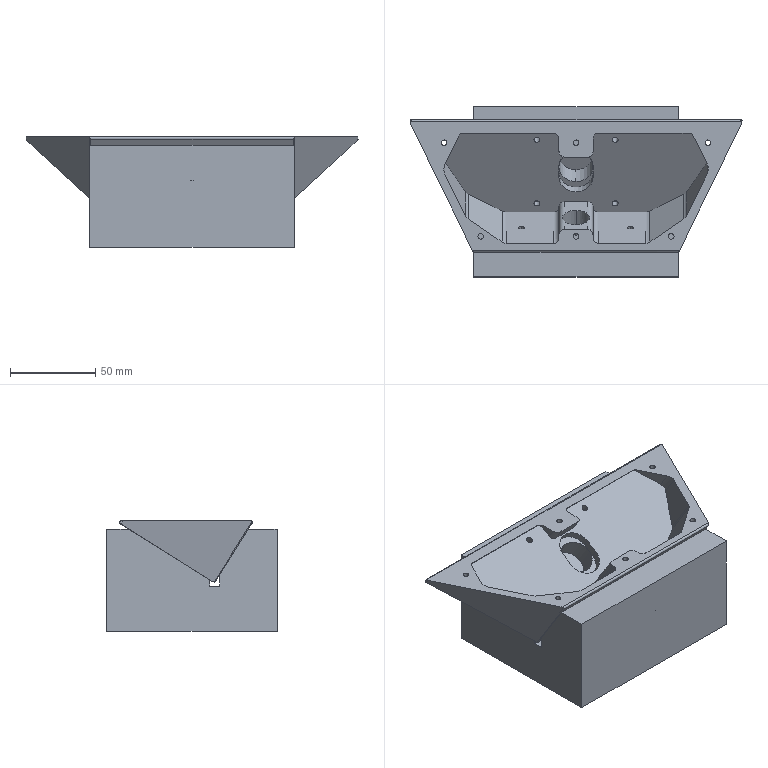NC program | Mastercam | posted with a generic post | part box 195.124 x 100 x 65 mm
Lines 1 to 1369 of 1918, first 1278 of 1369 lines:
%
O0000()
(MATERIAL - ALUMINUM MM - 2024)
( T1 | 16 RC | H1 | D1 | WEAR COMP | TOOL DIA. - 16. | XY STOCK TO LEAVE - -3. | Z STOCK TO LEAVE - .1 )
( T2 | 16 FI | H2 | D2 | WEAR COMP | TOOL DIA. - 16. | XY STOCK TO LEAVE - -3. | Z STOCK TO LEAVE - 0. )
( T3 | 6 SPD | H3 )
( T4 | 3.3 DR | H4 )
( T5 | 3.2 DR | H5 )
( T6 | 2.5 FEM | H6 | D6 | WEAR COMP | TOOL DIA. - 2.5 | XY STOCK TO LEAVE - -.015 | Z STOCK TO LEAVE - 0. )
( T7 | 3.15 THML | H7 | D7 | WEAR COMP | TOOL DIA. - 3.15 )
( T11 | 3.5 DR | H11 )
N100 G21
N110 G0 G17 G40 G49 G80 G90
N120 T1 M6
N130 G0 G90 G54 X-86.736 Y-13.812 A0. S2300 M3
N140 G43 H1 Z50.
N150 Z36.439
N160 G1 Z.1 F2000.
N170 G41 D1 X-75.958 Y-8.535 F3000.
N180 G3 X-75.509 Y-7.816 I-.352 J.719
N190 G1 X-75.53 Y-7.636
N200 X-75.591 Y-7.464
N210 X-81.561 Y4.728
N220 X-82.05 Y5.913
N230 X-82.43 Y7.304
N240 X-82.637 Y8.729
N250 X-82.672 Y10.164
N260 X-82.534 Y11.588
N270 X-82.229 Y12.977
N280 X-81.788 Y14.23
N290 X-81.522 Y14.815
N300 X-73.284 Y31.64
N310 X-72.634 Y32.725
N320 X-71.667 Y33.84
N330 X-70.515 Y34.764
N340 X-69.209 Y35.459
N350 X-67.795 Y35.893
N360 X-66.565 Y36.019
N370 X-12.744 Y36.02
N380 X-11.467 Y35.889
N390 X-10.017 Y35.434
N400 X-8.708 Y34.72
N410 X-7.575 Y33.794
N420 X-6.639 Y32.702
N430 X-5.911 Y31.486
N440 X-5.393 Y30.185
N450 X-5.086 Y28.835
N460 X-5. Y27.667
N470 Y21.868
N480 X5.
N490 Y27.683
N500 X5.102 Y28.951
N510 X5.452 Y30.375
N520 X6.028 Y31.717
N530 X6.817 Y32.942
N540 X7.807 Y34.013
N550 X8.974 Y34.891
N560 X10.285 Y35.541
N570 X11.67 Y35.923
N580 X12.783 Y36.02
N590 X66.704
N600 X67.965 Y35.892
N610 X69.4 Y35.448
N620 X70.699 Y34.749
N630 X71.827 Y33.841
N640 X72.762 Y32.769
N650 X73.401 Y31.728
N660 X81.643 Y14.901
N670 X82.132 Y13.716
N680 X82.512 Y12.324
N690 X82.719 Y10.899
N700 X82.753 Y9.464
N710 X82.616 Y8.04
N720 X82.31 Y6.651
N730 X81.87 Y5.399
N740 X81.603 Y4.813
N750 X69.621 Y-19.658
N760 X68.987 Y-20.768
N770 X68.12 Y-21.904
N780 X67.136 Y-22.885
N790 X66.307 Y-23.523
N800 X46.099 Y-37.28
N810 X45.017 Y-37.907
N820 X43.691 Y-38.431
N830 X42.312 Y-38.746
N840 X41.122 Y-38.835
N850 X12.744
N860 X11.467 Y-38.703
N870 X10.017 Y-38.248
N880 X8.708 Y-37.535
N890 X7.575 Y-36.609
N900 X6.639 Y-35.517
N910 X5.911 Y-34.301
N920 X5.393 Y-33.
N930 X5.086 Y-31.65
N940 X5.007 Y-30.58
N950 X-5.007
N960 X-5.102 Y-31.766
N970 X-5.452 Y-33.189
N980 X-6.028 Y-34.531
N990 X-6.817 Y-35.756
N1000 X-7.807 Y-36.827
N1010 X-8.974 Y-37.706
N1020 X-10.285 Y-38.355
N1030 X-11.67 Y-38.738
N1040 X-12.783 Y-38.835
N1050 X-41.13
N1060 X-42.359 Y-38.739
N1070 X-43.741 Y-38.415
N1080 X-45.049 Y-37.891
N1090 X-46.104 Y-37.278
N1100 X-66.333 Y-23.505
N1110 X-67.302 Y-22.739
N1120 X-68.278 Y-21.718
N1130 X-69.095 Y-20.598
N1140 X-69.633 Y-19.636
N1150 X-75.812 Y-7.016
N1160 G3 X-76.53 Y-6.568 I-.718 J-.351
N1170 X-76.882 Y-6.649 I0. J-.799
N1180 G1 G40 X-87.659 Y-11.926
N1190 G0 Z50.
N1200 X-63.18 Y.421
N1210 Z36.439
N1220 G1 Z.1 F2000.
N1230 G41 D1 X-73.958 Y-4.856 F3000.
N1240 G3 X-74.406 Y-5.574 I.352 J-.718
N1250 X-74.325 Y-5.926 I.8 J0.
N1260 G1 X-59.636 Y-35.926
N1270 X59.636
N1280 X94.816 Y35.926
N1290 X-94.816
N1300 X-74.105 Y-6.375
N1310 G3 X-73.386 Y-6.824 I.719 J.352
N1320 X-73.034 Y-6.742 I0. J.801
N1330 G1 G40 X-62.257 Y-1.465
N1340 G0 Z50.
N1350 M5
N1360 G91 G28 Z0.
N1370 A0.
N1380 M01
N1390 T2 M6
N1400 G0 G90 G17 G54 X-86.736 Y-13.812 A0. S4000 M3
N1410 G43 H2 Z50.
N1420 Z36.439
N1430 G1 Z0. F2000.
N1440 G41 D2 X-75.958 Y-8.535 F800.
N1450 G3 X-75.509 Y-7.816 I-.352 J.719
N1460 G1 X-75.53 Y-7.636
N1470 X-75.591 Y-7.464
N1480 X-81.561 Y4.728
N1490 X-82.05 Y5.913
N1500 X-82.43 Y7.304
N1510 X-82.637 Y8.729
N1520 X-82.672 Y10.164
N1530 X-82.534 Y11.588
N1540 X-82.229 Y12.977
N1550 X-81.788 Y14.23
N1560 X-81.522 Y14.815
N1570 X-73.284 Y31.64
N1580 X-72.634 Y32.725
N1590 X-71.667 Y33.84
N1600 X-70.515 Y34.764
N1610 X-69.209 Y35.459
N1620 X-67.795 Y35.893
N1630 X-66.565 Y36.019
N1640 X-12.744 Y36.02
N1650 X-11.467 Y35.889
N1660 X-10.017 Y35.434
N1670 X-8.708 Y34.72
N1680 X-7.575 Y33.794
N1690 X-6.639 Y32.702
N1700 X-5.911 Y31.486
N1710 X-5.393 Y30.185
N1720 X-5.086 Y28.835
N1730 X-5. Y27.667
N1740 Y21.868
N1750 X5.
N1760 Y27.683
N1770 X5.102 Y28.951
N1780 X5.452 Y30.375
N1790 X6.028 Y31.717
N1800 X6.817 Y32.942
N1810 X7.807 Y34.013
N1820 X8.974 Y34.891
N1830 X10.285 Y35.541
N1840 X11.67 Y35.923
N1850 X12.783 Y36.02
N1860 X66.704
N1870 X67.965 Y35.892
N1880 X69.4 Y35.448
N1890 X70.699 Y34.749
N1900 X71.827 Y33.841
N1910 X72.762 Y32.769
N1920 X73.401 Y31.728
N1930 X81.643 Y14.901
N1940 X82.132 Y13.716
N1950 X82.512 Y12.324
N1960 X82.719 Y10.899
N1970 X82.753 Y9.464
N1980 X82.616 Y8.04
N1990 X82.31 Y6.651
N2000 X81.87 Y5.399
N2010 X81.603 Y4.813
N2020 X69.621 Y-19.658
N2030 X68.987 Y-20.768
N2040 X68.12 Y-21.904
N2050 X67.136 Y-22.885
N2060 X66.307 Y-23.523
N2070 X46.099 Y-37.28
N2080 X45.017 Y-37.907
N2090 X43.691 Y-38.431
N2100 X42.312 Y-38.746
N2110 X41.122 Y-38.835
N2120 X12.744
N2130 X11.467 Y-38.703
N2140 X10.017 Y-38.248
N2150 X8.708 Y-37.535
N2160 X7.575 Y-36.609
N2170 X6.639 Y-35.517
N2180 X5.911 Y-34.301
N2190 X5.393 Y-33.
N2200 X5.086 Y-31.65
N2210 X5.007 Y-30.58
N2220 X-5.007
N2230 X-5.102 Y-31.766
N2240 X-5.452 Y-33.189
N2250 X-6.028 Y-34.531
N2260 X-6.817 Y-35.756
N2270 X-7.807 Y-36.827
N2280 X-8.974 Y-37.706
N2290 X-10.285 Y-38.355
N2300 X-11.67 Y-38.738
N2310 X-12.783 Y-38.835
N2320 X-41.13
N2330 X-42.359 Y-38.739
N2340 X-43.741 Y-38.415
N2350 X-45.049 Y-37.891
N2360 X-46.104 Y-37.278
N2370 X-66.333 Y-23.505
N2380 X-67.302 Y-22.739
N2390 X-68.278 Y-21.718
N2400 X-69.095 Y-20.598
N2410 X-69.633 Y-19.636
N2420 X-75.812 Y-7.016
N2430 G3 X-76.53 Y-6.568 I-.718 J-.351
N2440 X-76.882 Y-6.649 I0. J-.799
N2450 G1 G40 X-87.659 Y-11.926
N2460 G0 Z50.
N2470 X-63.18 Y.421
N2480 Z36.439
N2490 G1 Z0. F2000.
N2500 G41 D2 X-73.958 Y-4.856 F800.
N2510 G3 X-74.406 Y-5.574 I.352 J-.718
N2520 X-74.325 Y-5.926 I.8 J0.
N2530 G1 X-59.636 Y-35.926
N2540 X59.636
N2550 X94.816 Y35.926
N2560 X-94.816
N2570 X-74.105 Y-6.375
N2580 G3 X-73.386 Y-6.824 I.719 J.352
N2590 X-73.034 Y-6.742 I0. J.801
N2600 G1 G40 X-62.257 Y-1.465
N2610 G0 Z50.
N2620 M5
N2630 G91 G28 Z0.
N2640 A0.
N2650 M01
N2660 T3 M6
N2670 G0 G90 G17 G54 X77.5 Y25.269 A0. S2000 M3
N2680 G43 H3 Z50.
N2690 G98 G81 Z-2. R1. F100.
N2700 X0.
N2710 X-77.5
N2720 X-56. Y-29.731
N2730 X0.
N2740 X56.
N2750 G80
N2760 M5
N2770 G91 G0 G28 Z0.
N2780 A0.
N2790 M01
N2800 T4 M6
N2810 G0 G90 G17 G54 X56. Y-29.731 A0. S1200 M3
N2820 G43 H4 Z50.
N2830 G98 G83 Z-8. R1. Q3. F100.
N2840 X-56.
N2850 G80
N2860 G0 X77.5 Y25.269
N2870 G98 G83 Z-7.5 R1. Q3. F100.
N2880 X-77.5
N2890 G80
N2900 M5
N2910 G91 G0 G28 Z0.
N2920 A0.
N2930 M01
N2940 T5 M6
N2950 G0 G90 G17 G54 X0. Y-29.731 A0. S1200 M3
N2960 G43 H5 Z50.
N2970 G98 G81 Z-8. R1. F100.
N2980 Y25.269
N2990 G80
N3000 G0 Y-29.731
N3010 G98 G81 Z-8. R1. F100.
N3020 Y25.269
N3030 G80
N3040 M5
N3050 G91 G0 G28 Z0.
N3060 A0.
N3070 M01
N3080 T6 M6
N3090 G0 G90 G17 G54 X0. Y-29.731 A0. S3500 M3
N3100 G43 H6 Z50.
N3110 Z2.
N3120 G1 Z-6. F600.
N3130 G41 D6 X.39 F100.
N3140 G3 X.403 Y-29.66 I-.195 J.071
N3150 X.39 Y-29.589 I-.208 J0.
N3160 X0. Y-29.316 I-.39 J-.142
N3170 X-.415 Y-29.731 I0. J-.415
N3180 X0. Y-30.146 I.415 J0.
N3190 X.415 Y-29.731 I0. J.415
N3200 X.39 Y-29.589 I-.415 J0.
N3210 X.331 Y-29.48 I-.39 J-.142
N3220 X.211 Y-29.403 I-.166 J-.125
N3230 G1 G40 X0. Y-29.731
N3240 G41 D6 X.39
N3250 G3 X.403 Y-29.66 I-.195 J.071
N3260 X.39 Y-29.589 I-.208 J0.
N3270 X0. Y-29.316 I-.39 J-.142
N3280 X-.415 Y-29.731 I0. J-.415
N3290 X0. Y-30.146 I.415 J0.
N3300 X.415 Y-29.731 I0. J.415
N3310 X.39 Y-29.589 I-.415 J0.
N3320 X.331 Y-29.48 I-.39 J-.142
N3330 X.211 Y-29.403 I-.166 J-.125
N3340 G1 G40 X0. Y-29.731
N3350 G0 Z50.
N3360 Y25.269
N3370 Z2.
N3380 G1 Z-6. F600.
N3390 G41 D6 X.39 F100.
N3400 G3 X.403 Y25.34 I-.195 J.071
N3410 X.39 Y25.411 I-.208 J0.
N3420 X0. Y25.684 I-.39 J-.142
N3430 X-.415 Y25.269 I0. J-.415
N3440 X0. Y24.854 I.415 J0.
N3450 X.415 Y25.269 I0. J.415
N3460 X.39 Y25.411 I-.415 J0.
N3470 X.331 Y25.52 I-.39 J-.142
N3480 X.211 Y25.597 I-.166 J-.125
N3490 G1 G40 X0. Y25.269
N3500 G41 D6 X.39
N3510 G3 X.403 Y25.34 I-.195 J.071
N3520 X.39 Y25.411 I-.208 J0.
N3530 X0. Y25.684 I-.39 J-.142
N3540 X-.415 Y25.269 I0. J-.415
N3550 X0. Y24.854 I.415 J0.
N3560 X.415 Y25.269 I0. J.415
N3570 X.39 Y25.411 I-.415 J0.
N3580 X.331 Y25.52 I-.39 J-.142
N3590 X.211 Y25.597 I-.166 J-.125
N3600 G1 G40 X0. Y25.269
N3610 G0 Z50.
N3620 M5
N3630 G91 G28 Z0.
N3640 A0.
N3650 M01
N3660 T7 M6
N3670 G0 G90 G17 G54 X56. Y-29.731 A0. S3000 M3
N3680 G43 H7 Z50.
N3690 Z2.
N3700 G1 Z-5.5 F600.
N3710 G41 D7 Y-29.891 F200.
N3720 G3 X56.16 Y-29.731 Z-5.325 I0. J.16
N3730 X56. Y-29.571 Z-5.15 I-.16 J0.
N3740 X55.84 Y-29.731 Z-4.975 I0. J-.16
N3750 X56. Y-29.891 Z-4.8 I.16 J0.
N3760 X56.16 Y-29.731 Z-4.625 I0. J.16
N3770 X56. Y-29.571 Z-4.45 I-.16 J0.
N3780 G1 G40 Y-29.731
N3790 Z-3.4 F600.
N3800 G41 D7 Y-29.891 F200.
N3810 G3 X56.16 Y-29.731 Z-3.225 I0. J.16
N3820 X56. Y-29.571 Z-3.05 I-.16 J0.
N3830 X55.84 Y-29.731 Z-2.875 I0. J-.16
N3840 X56. Y-29.891 Z-2.7 I.16 J0.
N3850 X56.16 Y-29.731 Z-2.525 I0. J.16
N3860 X56. Y-29.571 Z-2.35 I-.16 J0.
N3870 G1 G40 Y-29.731
N3880 Z-1.3 F600.
N3890 G41 D7 Y-29.891 F200.
N3900 G3 X56.16 Y-29.731 Z-1.125 I0. J.16
N3910 X56. Y-29.571 Z-.95 I-.16 J0.
N3920 X55.84 Y-29.731 Z-.775 I0. J-.16
N3930 X56. Y-29.891 Z-.6 I.16 J0.
N3940 X56.16 Y-29.731 Z-.425 I0. J.16
N3950 X56. Y-29.571 Z-.25 I-.16 J0.
N3960 G1 G40 Y-29.731
N3970 Z-5.5 F600.
N3980 G41 D7 Y-29.956 F200.
N3990 G3 X56.225 Y-29.731 Z-5.325 I0. J.225
N4000 X56. Y-29.506 Z-5.15 I-.225 J0.
N4010 X55.775 Y-29.731 Z-4.975 I0. J-.225
N4020 X56. Y-29.956 Z-4.8 I.225 J0.
N4030 X56.225 Y-29.731 Z-4.625 I0. J.225
N4040 X56. Y-29.506 Z-4.45 I-.225 J0.
N4050 G1 G40 Y-29.731
N4060 Z-3.4 F600.
N4070 G41 D7 Y-29.956 F200.
N4080 G3 X56.225 Y-29.731 Z-3.225 I0. J.225
N4090 X56. Y-29.506 Z-3.05 I-.225 J0.
N4100 X55.775 Y-29.731 Z-2.875 I0. J-.225
N4110 X56. Y-29.956 Z-2.7 I.225 J0.
N4120 X56.225 Y-29.731 Z-2.525 I0. J.225
N4130 X56. Y-29.506 Z-2.35 I-.225 J0.
N4140 G1 G40 Y-29.731
N4150 Z-1.3 F600.
N4160 G41 D7 Y-29.956 F200.
N4170 G3 X56.225 Y-29.731 Z-1.125 I0. J.225
N4180 X56. Y-29.506 Z-.95 I-.225 J0.
N4190 X55.775 Y-29.731 Z-.775 I0. J-.225
N4200 X56. Y-29.956 Z-.6 I.225 J0.
N4210 X56.225 Y-29.731 Z-.425 I0. J.225
N4220 X56. Y-29.506 Z-.25 I-.225 J0.
N4230 G1 G40 Y-29.731
N4240 Z-5.5 F600.
N4250 G41 D7 Y-30.021 F200.
N4260 G3 X56.29 Y-29.731 Z-5.325 I0. J.29
N4270 X56. Y-29.441 Z-5.15 I-.29 J0.
N4280 X55.71 Y-29.731 Z-4.975 I0. J-.29
N4290 X56. Y-30.021 Z-4.8 I.29 J0.
N4300 X56.29 Y-29.731 Z-4.625 I0. J.29
N4310 X56. Y-29.441 Z-4.45 I-.29 J0.
N4320 G1 G40 Y-29.731
N4330 Z-3.4 F600.
N4340 G41 D7 Y-30.021 F200.
N4350 G3 X56.29 Y-29.731 Z-3.225 I0. J.29
N4360 X56. Y-29.441 Z-3.05 I-.29 J0.
N4370 X55.71 Y-29.731 Z-2.875 I0. J-.29
N4380 X56. Y-30.021 Z-2.7 I.29 J0.
N4390 X56.29 Y-29.731 Z-2.525 I0. J.29
N4400 X56. Y-29.441 Z-2.35 I-.29 J0.
N4410 G1 G40 Y-29.731
N4420 Z-1.3 F600.
N4430 G41 D7 Y-30.021 F200.
N4440 G3 X56.29 Y-29.731 Z-1.125 I0. J.29
N4450 X56. Y-29.441 Z-.95 I-.29 J0.
N4460 X55.71 Y-29.731 Z-.775 I0. J-.29
N4470 X56. Y-30.021 Z-.6 I.29 J0.
N4480 X56.29 Y-29.731 Z-.425 I0. J.29
N4490 X56. Y-29.441 Z-.25 I-.29 J0.
N4500 G1 G40 Y-29.731
N4510 Z-5.5 F600.
N4520 G41 D7 Y-30.086 F200.
N4530 G3 X56.355 Y-29.731 Z-5.325 I0. J.355
N4540 X56. Y-29.376 Z-5.15 I-.355 J0.
N4550 X55.645 Y-29.731 Z-4.975 I0. J-.355
N4560 X56. Y-30.086 Z-4.8 I.355 J0.
N4570 X56.355 Y-29.731 Z-4.625 I0. J.355
N4580 X56. Y-29.376 Z-4.45 I-.355 J0.
N4590 G1 G40 Y-29.731
N4600 Z-3.4 F600.
N4610 G41 D7 Y-30.086 F200.
N4620 G3 X56.355 Y-29.731 Z-3.225 I0. J.355
N4630 X56. Y-29.376 Z-3.05 I-.355 J0.
N4640 X55.645 Y-29.731 Z-2.875 I0. J-.355
N4650 X56. Y-30.086 Z-2.7 I.355 J0.
N4660 X56.355 Y-29.731 Z-2.525 I0. J.355
N4670 X56. Y-29.376 Z-2.35 I-.355 J0.
N4680 G1 G40 Y-29.731
N4690 Z-1.3 F600.
N4700 G41 D7 Y-30.086 F200.
N4710 G3 X56.355 Y-29.731 Z-1.125 I0. J.355
N4720 X56. Y-29.376 Z-.95 I-.355 J0.
N4730 X55.645 Y-29.731 Z-.775 I0. J-.355
N4740 X56. Y-30.086 Z-.6 I.355 J0.
N4750 X56.355 Y-29.731 Z-.425 I0. J.355
N4760 X56. Y-29.376 Z-.25 I-.355 J0.
N4770 G1 G40 Y-29.731
N4780 Z-5.5 F600.
N4790 G41 D7 Y-30.151 F200.
N4800 G3 X56.42 Y-29.731 Z-5.325 I0. J.42
N4810 X56. Y-29.311 Z-5.15 I-.42 J0.
N4820 X55.58 Y-29.731 Z-4.975 I0. J-.42
N4830 X56. Y-30.151 Z-4.8 I.42 J0.
N4840 X56.42 Y-29.731 Z-4.625 I0. J.42
N4850 X56. Y-29.311 Z-4.45 I-.42 J0.
N4860 G1 G40 Y-29.731
N4870 Z-3.4 F600.
N4880 G41 D7 Y-30.151 F200.
N4890 G3 X56.42 Y-29.731 Z-3.225 I0. J.42
N4900 X56. Y-29.311 Z-3.05 I-.42 J0.
N4910 X55.58 Y-29.731 Z-2.875 I0. J-.42
N4920 X56. Y-30.151 Z-2.7 I.42 J0.
N4930 X56.42 Y-29.731 Z-2.525 I0. J.42
N4940 X56. Y-29.311 Z-2.35 I-.42 J0.
N4950 G1 G40 Y-29.731
N4960 Z-1.3 F600.
N4970 G41 D7 Y-30.151 F200.
N4980 G3 X56.42 Y-29.731 Z-1.125 I0. J.42
N4990 X56. Y-29.311 Z-.95 I-.42 J0.
N5000 X55.58 Y-29.731 Z-.775 I0. J-.42
N5010 X56. Y-30.151 Z-.6 I.42 J0.
N5020 X56.42 Y-29.731 Z-.425 I0. J.42
N5030 X56. Y-29.311 Z-.25 I-.42 J0.
N5040 G1 G40 Y-29.731
N5050 Z-5.5 F600.
N5060 G41 D7 Y-30.156 F200.
N5070 G3 X56.425 Y-29.731 Z-5.325 I0. J.425
N5080 X56. Y-29.306 Z-5.15 I-.425 J0.
N5090 X55.575 Y-29.731 Z-4.975 I0. J-.425
N5100 X56. Y-30.156 Z-4.8 I.425 J0.
N5110 X56.425 Y-29.731 Z-4.625 I0. J.425
N5120 X56. Y-29.306 Z-4.45 I-.425 J0.
N5130 G1 G40 Y-29.731
N5140 Z-3.4 F600.
N5150 G41 D7 Y-30.156 F200.
N5160 G3 X56.425 Y-29.731 Z-3.225 I0. J.425
N5170 X56. Y-29.306 Z-3.05 I-.425 J0.
N5180 X55.575 Y-29.731 Z-2.875 I0. J-.425
N5190 X56. Y-30.156 Z-2.7 I.425 J0.
N5200 X56.425 Y-29.731 Z-2.525 I0. J.425
N5210 X56. Y-29.306 Z-2.35 I-.425 J0.
N5220 G1 G40 Y-29.731
N5230 Z-1.3 F600.
N5240 G41 D7 Y-30.156 F200.
N5250 G3 X56.425 Y-29.731 Z-1.125 I0. J.425
N5260 X56. Y-29.306 Z-.95 I-.425 J0.
N5270 X55.575 Y-29.731 Z-.775 I0. J-.425
N5280 X56. Y-30.156 Z-.6 I.425 J0.
N5290 X56.425 Y-29.731 Z-.425 I0. J.425
N5300 X56. Y-29.306 Z-.25 I-.425 J0.
N5310 G1 G40 Y-29.731
N5320 G0 Z2.
N5330 Z50.
N5340 X0.
N5350 Z2.
N5360 G1 Z-5.5 F600.
N5370 G41 D7 Y-29.891 F200.
N5380 G3 X.16 Y-29.731 Z-5.325 I0. J.16
N5390 X0. Y-29.571 Z-5.15 I-.16 J0.
N5400 X-.16 Y-29.731 Z-4.975 I0. J-.16
N5410 X0. Y-29.891 Z-4.8 I.16 J0.
N5420 X.16 Y-29.731 Z-4.625 I0. J.16
N5430 X0. Y-29.571 Z-4.45 I-.16 J0.
N5440 G1 G40 Y-29.731
N5450 Z-3.4 F600.
N5460 G41 D7 Y-29.891 F200.
N5470 G3 X.16 Y-29.731 Z-3.225 I0. J.16
N5480 X0. Y-29.571 Z-3.05 I-.16 J0.
N5490 X-.16 Y-29.731 Z-2.875 I0. J-.16
N5500 X0. Y-29.891 Z-2.7 I.16 J0.
N5510 X.16 Y-29.731 Z-2.525 I0. J.16
N5520 X0. Y-29.571 Z-2.35 I-.16 J0.
N5530 G1 G40 Y-29.731
N5540 Z-1.3 F600.
N5550 G41 D7 Y-29.891 F200.
N5560 G3 X.16 Y-29.731 Z-1.125 I0. J.16
N5570 X0. Y-29.571 Z-.95 I-.16 J0.
N5580 X-.16 Y-29.731 Z-.775 I0. J-.16
N5590 X0. Y-29.891 Z-.6 I.16 J0.
N5600 X.16 Y-29.731 Z-.425 I0. J.16
N5610 X0. Y-29.571 Z-.25 I-.16 J0.
N5620 G1 G40 Y-29.731
N5630 Z-5.5 F600.
N5640 G41 D7 Y-29.956 F200.
N5650 G3 X.225 Y-29.731 Z-5.325 I0. J.225
N5660 X0. Y-29.506 Z-5.15 I-.225 J0.
N5670 X-.225 Y-29.731 Z-4.975 I0. J-.225
N5680 X0. Y-29.956 Z-4.8 I.225 J0.
N5690 X.225 Y-29.731 Z-4.625 I0. J.225
N5700 X0. Y-29.506 Z-4.45 I-.225 J0.
N5710 G1 G40 Y-29.731
N5720 Z-3.4 F600.
N5730 G41 D7 Y-29.956 F200.
N5740 G3 X.225 Y-29.731 Z-3.225 I0. J.225
N5750 X0. Y-29.506 Z-3.05 I-.225 J0.
N5760 X-.225 Y-29.731 Z-2.875 I0. J-.225
N5770 X0. Y-29.956 Z-2.7 I.225 J0.
N5780 X.225 Y-29.731 Z-2.525 I0. J.225
N5790 X0. Y-29.506 Z-2.35 I-.225 J0.
N5800 G1 G40 Y-29.731
N5810 Z-1.3 F600.
N5820 G41 D7 Y-29.956 F200.
N5830 G3 X.225 Y-29.731 Z-1.125 I0. J.225
N5840 X0. Y-29.506 Z-.95 I-.225 J0.
N5850 X-.225 Y-29.731 Z-.775 I0. J-.225
N5860 X0. Y-29.956 Z-.6 I.225 J0.
N5870 X.225 Y-29.731 Z-.425 I0. J.225
N5880 X0. Y-29.506 Z-.25 I-.225 J0.
N5890 G1 G40 Y-29.731
N5900 Z-5.5 F600.
N5910 G41 D7 Y-30.021 F200.
N5920 G3 X.29 Y-29.731 Z-5.325 I0. J.29
N5930 X0. Y-29.441 Z-5.15 I-.29 J0.
N5940 X-.29 Y-29.731 Z-4.975 I0. J-.29
N5950 X0. Y-30.021 Z-4.8 I.29 J0.
N5960 X.29 Y-29.731 Z-4.625 I0. J.29
N5970 X0. Y-29.441 Z-4.45 I-.29 J0.
N5980 G1 G40 Y-29.731
N5990 Z-3.4 F600.
N6000 G41 D7 Y-30.021 F200.
N6010 G3 X.29 Y-29.731 Z-3.225 I0. J.29
N6020 X0. Y-29.441 Z-3.05 I-.29 J0.
N6030 X-.29 Y-29.731 Z-2.875 I0. J-.29
N6040 X0. Y-30.021 Z-2.7 I.29 J0.
N6050 X.29 Y-29.731 Z-2.525 I0. J.29
N6060 X0. Y-29.441 Z-2.35 I-.29 J0.
N6070 G1 G40 Y-29.731
N6080 Z-1.3 F600.
N6090 G41 D7 Y-30.021 F200.
N6100 G3 X.29 Y-29.731 Z-1.125 I0. J.29
N6110 X0. Y-29.441 Z-.95 I-.29 J0.
N6120 X-.29 Y-29.731 Z-.775 I0. J-.29
N6130 X0. Y-30.021 Z-.6 I.29 J0.
N6140 X.29 Y-29.731 Z-.425 I0. J.29
N6150 X0. Y-29.441 Z-.25 I-.29 J0.
N6160 G1 G40 Y-29.731
N6170 Z-5.5 F600.
N6180 G41 D7 Y-30.086 F200.
N6190 G3 X.355 Y-29.731 Z-5.325 I0. J.355
N6200 X0. Y-29.376 Z-5.15 I-.355 J0.
N6210 X-.355 Y-29.731 Z-4.975 I0. J-.355
N6220 X0. Y-30.086 Z-4.8 I.355 J0.
N6230 X.355 Y-29.731 Z-4.625 I0. J.355
N6240 X0. Y-29.376 Z-4.45 I-.355 J0.
N6250 G1 G40 Y-29.731
N6260 Z-3.4 F600.
N6270 G41 D7 Y-30.086 F200.
N6280 G3 X.355 Y-29.731 Z-3.225 I0. J.355
N6290 X0. Y-29.376 Z-3.05 I-.355 J0.
N6300 X-.355 Y-29.731 Z-2.875 I0. J-.355
N6310 X0. Y-30.086 Z-2.7 I.355 J0.
N6320 X.355 Y-29.731 Z-2.525 I0. J.355
N6330 X0. Y-29.376 Z-2.35 I-.355 J0.
N6340 G1 G40 Y-29.731
N6350 Z-1.3 F600.
N6360 G41 D7 Y-30.086 F200.
N6370 G3 X.355 Y-29.731 Z-1.125 I0. J.355
N6380 X0. Y-29.376 Z-.95 I-.355 J0.
N6390 X-.355 Y-29.731 Z-.775 I0. J-.355
N6400 X0. Y-30.086 Z-.6 I.355 J0.
N6410 X.355 Y-29.731 Z-.425 I0. J.355
N6420 X0. Y-29.376 Z-.25 I-.355 J0.
N6430 G1 G40 Y-29.731
N6440 Z-5.5 F600.
N6450 G41 D7 Y-30.151 F200.
N6460 G3 X.42 Y-29.731 Z-5.325 I0. J.42
N6470 X0. Y-29.311 Z-5.15 I-.42 J0.
N6480 X-.42 Y-29.731 Z-4.975 I0. J-.42
N6490 X0. Y-30.151 Z-4.8 I.42 J0.
N6500 X.42 Y-29.731 Z-4.625 I0. J.42
N6510 X0. Y-29.311 Z-4.45 I-.42 J0.
N6520 G1 G40 Y-29.731
N6530 Z-3.4 F600.
N6540 G41 D7 Y-30.151 F200.
N6550 G3 X.42 Y-29.731 Z-3.225 I0. J.42
N6560 X0. Y-29.311 Z-3.05 I-.42 J0.
N6570 X-.42 Y-29.731 Z-2.875 I0. J-.42
N6580 X0. Y-30.151 Z-2.7 I.42 J0.
N6590 X.42 Y-29.731 Z-2.525 I0. J.42
N6600 X0. Y-29.311 Z-2.35 I-.42 J0.
N6610 G1 G40 Y-29.731
N6620 Z-1.3 F600.
N6630 G41 D7 Y-30.151 F200.
N6640 G3 X.42 Y-29.731 Z-1.125 I0. J.42
N6650 X0. Y-29.311 Z-.95 I-.42 J0.
N6660 X-.42 Y-29.731 Z-.775 I0. J-.42
N6670 X0. Y-30.151 Z-.6 I.42 J0.
N6680 X.42 Y-29.731 Z-.425 I0. J.42
N6690 X0. Y-29.311 Z-.25 I-.42 J0.
N6700 G1 G40 Y-29.731
N6710 Z-5.5 F600.
N6720 G41 D7 Y-30.156 F200.
N6730 G3 X.425 Y-29.731 Z-5.325 I0. J.425
N6740 X0. Y-29.306 Z-5.15 I-.425 J0.
N6750 X-.425 Y-29.731 Z-4.975 I0. J-.425
N6760 X0. Y-30.156 Z-4.8 I.425 J0.
N6770 X.425 Y-29.731 Z-4.625 I0. J.425
N6780 X0. Y-29.306 Z-4.45 I-.425 J0.
N6790 G1 G40 Y-29.731
N6800 Z-3.4 F600.
N6810 G41 D7 Y-30.156 F200.
N6820 G3 X.425 Y-29.731 Z-3.225 I0. J.425
N6830 X0. Y-29.306 Z-3.05 I-.425 J0.
N6840 X-.425 Y-29.731 Z-2.875 I0. J-.425
N6850 X0. Y-30.156 Z-2.7 I.425 J0.
N6860 X.425 Y-29.731 Z-2.525 I0. J.425
N6870 X0. Y-29.306 Z-2.35 I-.425 J0.
N6880 G1 G40 Y-29.731
N6890 Z-1.3 F600.
N6900 G41 D7 Y-30.156 F200.
N6910 G3 X.425 Y-29.731 Z-1.125 I0. J.425
N6920 X0. Y-29.306 Z-.95 I-.425 J0.
N6930 X-.425 Y-29.731 Z-.775 I0. J-.425
N6940 X0. Y-30.156 Z-.6 I.425 J0.
N6950 X.425 Y-29.731 Z-.425 I0. J.425
N6960 X0. Y-29.306 Z-.25 I-.425 J0.
N6970 G1 G40 Y-29.731
N6980 G0 Z2.
N6990 Z50.
N7000 X-56.
N7010 Z2.
N7020 G1 Z-5.5 F600.
N7030 G41 D7 Y-29.891 F200.
N7040 G3 X-55.84 Y-29.731 Z-5.325 I0. J.16
N7050 X-56. Y-29.571 Z-5.15 I-.16 J0.
N7060 X-56.16 Y-29.731 Z-4.975 I0. J-.16
N7070 X-56. Y-29.891 Z-4.8 I.16 J0.
N7080 X-55.84 Y-29.731 Z-4.625 I0. J.16
N7090 X-56. Y-29.571 Z-4.45 I-.16 J0.
N7100 G1 G40 Y-29.731
N7110 Z-3.4 F600.
N7120 G41 D7 Y-29.891 F200.
N7130 G3 X-55.84 Y-29.731 Z-3.225 I0. J.16
N7140 X-56. Y-29.571 Z-3.05 I-.16 J0.
N7150 X-56.16 Y-29.731 Z-2.875 I0. J-.16
N7160 X-56. Y-29.891 Z-2.7 I.16 J0.
N7170 X-55.84 Y-29.731 Z-2.525 I0. J.16
N7180 X-56. Y-29.571 Z-2.35 I-.16 J0.
N7190 G1 G40 Y-29.731
N7200 Z-1.3 F600.
N7210 G41 D7 Y-29.891 F200.
N7220 G3 X-55.84 Y-29.731 Z-1.125 I0. J.16
N7230 X-56. Y-29.571 Z-.95 I-.16 J0.
N7240 X-56.16 Y-29.731 Z-.775 I0. J-.16
N7250 X-56. Y-29.891 Z-.6 I.16 J0.
N7260 X-55.84 Y-29.731 Z-.425 I0. J.16
N7270 X-56. Y-29.571 Z-.25 I-.16 J0.
N7280 G1 G40 Y-29.731
N7290 Z-5.5 F600.
N7300 G41 D7 Y-29.956 F200.
N7310 G3 X-55.775 Y-29.731 Z-5.325 I0. J.225
N7320 X-56. Y-29.506 Z-5.15 I-.225 J0.
N7330 X-56.225 Y-29.731 Z-4.975 I0. J-.225
N7340 X-56. Y-29.956 Z-4.8 I.225 J0.
N7350 X-55.775 Y-29.731 Z-4.625 I0. J.225
N7360 X-56. Y-29.506 Z-4.45 I-.225 J0.
N7370 G1 G40 Y-29.731
N7380 Z-3.4 F600.
N7390 G41 D7 Y-29.956 F200.
N7400 G3 X-55.775 Y-29.731 Z-3.225 I0. J.225
N7410 X-56. Y-29.506 Z-3.05 I-.225 J0.
N7420 X-56.225 Y-29.731 Z-2.875 I0. J-.225
N7430 X-56. Y-29.956 Z-2.7 I.225 J0.
N7440 X-55.775 Y-29.731 Z-2.525 I0. J.225
N7450 X-56. Y-29.506 Z-2.35 I-.225 J0.
N7460 G1 G40 Y-29.731
N7470 Z-1.3 F600.
N7480 G41 D7 Y-29.956 F200.
N7490 G3 X-55.775 Y-29.731 Z-1.125 I0. J.225
N7500 X-56. Y-29.506 Z-.95 I-.225 J0.
N7510 X-56.225 Y-29.731 Z-.775 I0. J-.225
N7520 X-56. Y-29.956 Z-.6 I.225 J0.
N7530 X-55.775 Y-29.731 Z-.425 I0. J.225
N7540 X-56. Y-29.506 Z-.25 I-.225 J0.
N7550 G1 G40 Y-29.731
N7560 Z-5.5 F600.
N7570 G41 D7 Y-30.021 F200.
N7580 G3 X-55.71 Y-29.731 Z-5.325 I0. J.29
N7590 X-56. Y-29.441 Z-5.15 I-.29 J0.
N7600 X-56.29 Y-29.731 Z-4.975 I0. J-.29
N7610 X-56. Y-30.021 Z-4.8 I.29 J0.
N7620 X-55.71 Y-29.731 Z-4.625 I0. J.29
N7630 X-56. Y-29.441 Z-4.45 I-.29 J0.
N7640 G1 G40 Y-29.731
N7650 Z-3.4 F600.
N7660 G41 D7 Y-30.021 F200.
N7670 G3 X-55.71 Y-29.731 Z-3.225 I0. J.29
N7680 X-56. Y-29.441 Z-3.05 I-.29 J0.
N7690 X-56.29 Y-29.731 Z-2.875 I0. J-.29
N7700 X-56. Y-30.021 Z-2.7 I.29 J0.
N7710 X-55.71 Y-29.731 Z-2.525 I0. J.29
N7720 X-56. Y-29.441 Z-2.35 I-.29 J0.
N7730 G1 G40 Y-29.731
N7740 Z-1.3 F600.
N7750 G41 D7 Y-30.021 F200.
N7760 G3 X-55.71 Y-29.731 Z-1.125 I0. J.29
N7770 X-56. Y-29.441 Z-.95 I-.29 J0.
N7780 X-56.29 Y-29.731 Z-.775 I0. J-.29
N7790 X-56. Y-30.021 Z-.6 I.29 J0.
N7800 X-55.71 Y-29.731 Z-.425 I0. J.29
N7810 X-56. Y-29.441 Z-.25 I-.29 J0.
N7820 G1 G40 Y-29.731
N7830 Z-5.5 F600.
N7840 G41 D7 Y-30.086 F200.
N7850 G3 X-55.645 Y-29.731 Z-5.325 I0. J.355
N7860 X-56. Y-29.376 Z-5.15 I-.355 J0.
N7870 X-56.355 Y-29.731 Z-4.975 I0. J-.355
N7880 X-56. Y-30.086 Z-4.8 I.355 J0.
N7890 X-55.645 Y-29.731 Z-4.625 I0. J.355
N7900 X-56. Y-29.376 Z-4.45 I-.355 J0.
N7910 G1 G40 Y-29.731
N7920 Z-3.4 F600.
N7930 G41 D7 Y-30.086 F200.
N7940 G3 X-55.645 Y-29.731 Z-3.225 I0. J.355
N7950 X-56. Y-29.376 Z-3.05 I-.355 J0.
N7960 X-56.355 Y-29.731 Z-2.875 I0. J-.355
N7970 X-56. Y-30.086 Z-2.7 I.355 J0.
N7980 X-55.645 Y-29.731 Z-2.525 I0. J.355
N7990 X-56. Y-29.376 Z-2.35 I-.355 J0.
N8000 G1 G40 Y-29.731
N8010 Z-1.3 F600.
N8020 G41 D7 Y-30.086 F200.
N8030 G3 X-55.645 Y-29.731 Z-1.125 I0. J.355
N8040 X-56. Y-29.376 Z-.95 I-.355 J0.
N8050 X-56.355 Y-29.731 Z-.775 I0. J-.355
N8060 X-56. Y-30.086 Z-.6 I.355 J0.
N8070 X-55.645 Y-29.731 Z-.425 I0. J.355
N8080 X-56. Y-29.376 Z-.25 I-.355 J0.
N8090 G1 G40 Y-29.731
N8100 Z-5.5 F600.
N8110 G41 D7 Y-30.151 F200.
N8120 G3 X-55.58 Y-29.731 Z-5.325 I0. J.42
N8130 X-56. Y-29.311 Z-5.15 I-.42 J0.
N8140 X-56.42 Y-29.731 Z-4.975 I0. J-.42
N8150 X-56. Y-30.151 Z-4.8 I.42 J0.
N8160 X-55.58 Y-29.731 Z-4.625 I0. J.42
N8170 X-56. Y-29.311 Z-4.45 I-.42 J0.
N8180 G1 G40 Y-29.731
N8190 Z-3.4 F600.
N8200 G41 D7 Y-30.151 F200.
N8210 G3 X-55.58 Y-29.731 Z-3.225 I0. J.42
N8220 X-56. Y-29.311 Z-3.05 I-.42 J0.
N8230 X-56.42 Y-29.731 Z-2.875 I0. J-.42
N8240 X-56. Y-30.151 Z-2.7 I.42 J0.
N8250 X-55.58 Y-29.731 Z-2.525 I0. J.42
N8260 X-56. Y-29.311 Z-2.35 I-.42 J0.
N8270 G1 G40 Y-29.731
N8280 Z-1.3 F600.
N8290 G41 D7 Y-30.151 F200.
N8300 G3 X-55.58 Y-29.731 Z-1.125 I0. J.42
N8310 X-56. Y-29.311 Z-.95 I-.42 J0.
N8320 X-56.42 Y-29.731 Z-.775 I0. J-.42
N8330 X-56. Y-30.151 Z-.6 I.42 J0.
N8340 X-55.58 Y-29.731 Z-.425 I0. J.42
N8350 X-56. Y-29.311 Z-.25 I-.42 J0.
N8360 G1 G40 Y-29.731
N8370 Z-5.5 F600.
N8380 G41 D7 Y-30.156 F200.
N8390 G3 X-55.575 Y-29.731 Z-5.325 I0. J.425
N8400 X-56. Y-29.306 Z-5.15 I-.425 J0.
N8410 X-56.425 Y-29.731 Z-4.975 I0. J-.425
N8420 X-56. Y-30.156 Z-4.8 I.425 J0.
N8430 X-55.575 Y-29.731 Z-4.625 I0. J.425
N8440 X-56. Y-29.306 Z-4.45 I-.425 J0.
N8450 G1 G40 Y-29.731
N8460 Z-3.4 F600.
N8470 G41 D7 Y-30.156 F200.
N8480 G3 X-55.575 Y-29.731 Z-3.225 I0. J.425
N8490 X-56. Y-29.306 Z-3.05 I-.425 J0.
N8500 X-56.425 Y-29.731 Z-2.875 I0. J-.425
N8510 X-56. Y-30.156 Z-2.7 I.425 J0.
N8520 X-55.575 Y-29.731 Z-2.525 I0. J.425
N8530 X-56. Y-29.306 Z-2.35 I-.425 J0.
N8540 G1 G40 Y-29.731
N8550 Z-1.3 F600.
N8560 G41 D7 Y-30.156 F200.
N8570 G3 X-55.575 Y-29.731 Z-1.125 I0. J.425
N8580 X-56. Y-29.306 Z-.95 I-.425 J0.
N8590 X-56.425 Y-29.731 Z-.775 I0. J-.425
N8600 X-56. Y-30.156 Z-.6 I.425 J0.
N8610 X-55.575 Y-29.731 Z-.425 I0. J.425
N8620 X-56. Y-29.306 Z-.25 I-.425 J0.
N8630 G1 G40 Y-29.731
N8640 G0 Z2.
N8650 Z50.
N8660 X-77.5 Y25.269
N8670 Z2.
N8680 G1 Z-5.5 F600.
N8690 G41 D7 Y25.109 F200.
N8700 G3 X-77.34 Y25.269 Z-5.325 I0. J.16
N8710 X-77.5 Y25.429 Z-5.15 I-.16 J0.
N8720 X-77.66 Y25.269 Z-4.975 I0. J-.16
N8730 X-77.5 Y25.109 Z-4.8 I.16 J0.
N8740 X-77.34 Y25.269 Z-4.625 I0. J.16
N8750 X-77.5 Y25.429 Z-4.45 I-.16 J0.
N8760 G1 G40 Y25.269
N8770 Z-3.4 F600.
N8780 G41 D7 Y25.109 F200.
N8790 G3 X-77.34 Y25.269 Z-3.225 I0. J.16
N8800 X-77.5 Y25.429 Z-3.05 I-.16 J0.
N8810 X-77.66 Y25.269 Z-2.875 I0. J-.16
N8820 X-77.5 Y25.109 Z-2.7 I.16 J0.
N8830 X-77.34 Y25.269 Z-2.525 I0. J.16
N8840 X-77.5 Y25.429 Z-2.35 I-.16 J0.
N8850 G1 G40 Y25.269
N8860 Z-1.3 F600.
N8870 G41 D7 Y25.109 F200.
N8880 G3 X-77.34 Y25.269 Z-1.125 I0. J.16
N8890 X-77.5 Y25.429 Z-.95 I-.16 J0.
N8900 X-77.66 Y25.269 Z-.775 I0. J-.16
N8910 X-77.5 Y25.109 Z-.6 I.16 J0.
N8920 X-77.34 Y25.269 Z-.425 I0. J.16
N8930 X-77.5 Y25.429 Z-.25 I-.16 J0.
N8940 G1 G40 Y25.269
N8950 Z-5.5 F600.
N8960 G41 D7 Y25.044 F200.
N8970 G3 X-77.275 Y25.269 Z-5.325 I0. J.225
N8980 X-77.5 Y25.494 Z-5.15 I-.225 J0.
N8990 X-77.725 Y25.269 Z-4.975 I0. J-.225
N9000 X-77.5 Y25.044 Z-4.8 I.225 J0.
N9010 X-77.275 Y25.269 Z-4.625 I0. J.225
N9020 X-77.5 Y25.494 Z-4.45 I-.225 J0.
N9030 G1 G40 Y25.269
N9040 Z-3.4 F600.
N9050 G41 D7 Y25.044 F200.
N9060 G3 X-77.275 Y25.269 Z-3.225 I0. J.225
N9070 X-77.5 Y25.494 Z-3.05 I-.225 J0.
N9080 X-77.725 Y25.269 Z-2.875 I0. J-.225
N9090 X-77.5 Y25.044 Z-2.7 I.225 J0.
N9100 X-77.275 Y25.269 Z-2.525 I0. J.225
N9110 X-77.5 Y25.494 Z-2.35 I-.225 J0.
N9120 G1 G40 Y25.269
N9130 Z-1.3 F600.
N9140 G41 D7 Y25.044 F200.
N9150 G3 X-77.275 Y25.269 Z-1.125 I0. J.225
N9160 X-77.5 Y25.494 Z-.95 I-.225 J0.
N9170 X-77.725 Y25.269 Z-.775 I0. J-.225
N9180 X-77.5 Y25.044 Z-.6 I.225 J0.
N9190 X-77.275 Y25.269 Z-.425 I0. J.225
N9200 X-77.5 Y25.494 Z-.25 I-.225 J0.
N9210 G1 G40 Y25.269
N9220 Z-5.5 F600.
N9230 G41 D7 Y24.979 F200.
N9240 G3 X-77.21 Y25.269 Z-5.325 I0. J.29
N9250 X-77.5 Y25.559 Z-5.15 I-.29 J0.
N9260 X-77.79 Y25.269 Z-4.975 I0. J-.29
N9270 X-77.5 Y24.979 Z-4.8 I.29 J0.
N9280 X-77.21 Y25.269 Z-4.625 I0. J.29
N9290 X-77.5 Y25.559 Z-4.45 I-.29 J0.
N9300 G1 G40 Y25.269
N9310 Z-3.4 F600.
N9320 G41 D7 Y24.979 F200.
N9330 G3 X-77.21 Y25.269 Z-3.225 I0. J.29
N9340 X-77.5 Y25.559 Z-3.05 I-.29 J0.
N9350 X-77.79 Y25.269 Z-2.875 I0. J-.29
N9360 X-77.5 Y24.979 Z-2.7 I.29 J0.
N9370 X-77.21 Y25.269 Z-2.525 I0. J.29
N9380 X-77.5 Y25.559 Z-2.35 I-.29 J0.
N9390 G1 G40 Y25.269
N9400 Z-1.3 F600.
N9410 G41 D7 Y24.979 F200.
N9420 G3 X-77.21 Y25.269 Z-1.125 I0. J.29
N9430 X-77.5 Y25.559 Z-.95 I-.29 J0.
N9440 X-77.79 Y25.269 Z-.775 I0. J-.29
N9450 X-77.5 Y24.979 Z-.6 I.29 J0.
N9460 X-77.21 Y25.269 Z-.425 I0. J.29
N9470 X-77.5 Y25.559 Z-.25 I-.29 J0.
N9480 G1 G40 Y25.269
N9490 Z-5.5 F600.
N9500 G41 D7 Y24.914 F200.
N9510 G3 X-77.145 Y25.269 Z-5.325 I0. J.355
N9520 X-77.5 Y25.624 Z-5.15 I-.355 J0.
N9530 X-77.855 Y25.269 Z-4.975 I0. J-.355
N9540 X-77.5 Y24.914 Z-4.8 I.355 J0.
N9550 X-77.145 Y25.269 Z-4.625 I0. J.355
N9560 X-77.5 Y25.624 Z-4.45 I-.355 J0.
N9570 G1 G40 Y25.269
N9580 Z-3.4 F600.
N9590 G41 D7 Y24.914 F200.
N9600 G3 X-77.145 Y25.269 Z-3.225 I0. J.355
N9610 X-77.5 Y25.624 Z-3.05 I-.355 J0.
N9620 X-77.855 Y25.269 Z-2.875 I0. J-.355
N9630 X-77.5 Y24.914 Z-2.7 I.355 J0.
N9640 X-77.145 Y25.269 Z-2.525 I0. J.355
N9650 X-77.5 Y25.624 Z-2.35 I-.355 J0.
N9660 G1 G40 Y25.269
N9670 Z-1.3 F600.
N9680 G41 D7 Y24.914 F200.
N9690 G3 X-77.145 Y25.269 Z-1.125 I0. J.355
N9700 X-77.5 Y25.624 Z-.95 I-.355 J0.
N9710 X-77.855 Y25.269 Z-.775 I0. J-.355
N9720 X-77.5 Y24.914 Z-.6 I.355 J0.
N9730 X-77.145 Y25.269 Z-.425 I0. J.355
N9740 X-77.5 Y25.624 Z-.25 I-.355 J0.
N9750 G1 G40 Y25.269
N9760 Z-5.5 F600.
N9770 G41 D7 Y24.849 F200.
N9780 G3 X-77.08 Y25.269 Z-5.325 I0. J.42
N9790 X-77.5 Y25.689 Z-5.15 I-.42 J0.
N9800 X-77.92 Y25.269 Z-4.975 I0. J-.42
N9810 X-77.5 Y24.849 Z-4.8 I.42 J0.
N9820 X-77.08 Y25.269 Z-4.625 I0. J.42
N9830 X-77.5 Y25.689 Z-4.45 I-.42 J0.
N9840 G1 G40 Y25.269
N9850 Z-3.4 F600.
N9860 G41 D7 Y24.849 F200.
N9870 G3 X-77.08 Y25.269 Z-3.225 I0. J.42
N9880 X-77.5 Y25.689 Z-3.05 I-.42 J0.
N9890 X-77.92 Y25.269 Z-2.875 I0. J-.42
N9900 X-77.5 Y24.849 Z-2.7 I.42 J0.
N9910 X-77.08 Y25.269 Z-2.525 I0. J.42
N9920 X-77.5 Y25.689 Z-2.35 I-.42 J0.
N9930 G1 G40 Y25.269
N9940 Z-1.3 F600.
N9950 G41 D7 Y24.849 F200.
N9960 G3 X-77.08 Y25.269 Z-1.125 I0. J.42
N9970 X-77.5 Y25.689 Z-.95 I-.42 J0.
N9980 X-77.92 Y25.269 Z-.775 I0. J-.42
N9990 X-77.5 Y24.849 Z-.6 I.42 J0.
N100 X-77.08 Y25.269 Z-.425 I0. J.42
N110 X-77.5 Y25.689 Z-.25 I-.42 J0.
N120 G1 G40 Y25.269
N130 Z-5.5 F600.
N140 G41 D7 Y24.844 F200.
N150 G3 X-77.075 Y25.269 Z-5.325 I0. J.425
N160 X-77.5 Y25.694 Z-5.15 I-.425 J0.
N170 X-77.925 Y25.269 Z-4.975 I0. J-.425
N180 X-77.5 Y24.844 Z-4.8 I.425 J0.
N190 X-77.075 Y25.269 Z-4.625 I0. J.425
N200 X-77.5 Y25.694 Z-4.45 I-.425 J0.
N210 G1 G40 Y25.269
N220 Z-3.4 F600.
N230 G41 D7 Y24.844 F200.
N240 G3 X-77.075 Y25.269 Z-3.225 I0. J.425
N250 X-77.5 Y25.694 Z-3.05 I-.425 J0.
N260 X-77.925 Y25.269 Z-2.875 I0. J-.425
N270 X-77.5 Y24.844 Z-2.7 I.425 J0.
N280 X-77.075 Y25.269 Z-2.525 I0. J.425
N290 X-77.5 Y25.694 Z-2.35 I-.425 J0.
N300 G1 G40 Y25.269
N310 Z-1.3 F600.
N320 G41 D7 Y24.844 F200.
N330 G3 X-77.075 Y25.269 Z-1.125 I0. J.425
N340 X-77.5 Y25.694 Z-.95 I-.425 J0.
N350 X-77.925 Y25.269 Z-.775 I0. J-.425
N360 X-77.5 Y24.844 Z-.6 I.425 J0.
N370 X-77.075 Y25.269 Z-.425 I0. J.425
N380 X-77.5 Y25.694 Z-.25 I-.425 J0.
N390 G1 G40 Y25.269
N400 G0 Z2.
N410 Z50.
N420 X0.
N430 Z2.
N440 G1 Z-5.5 F600.
N450 G41 D7 Y25.109 F200.
N460 G3 X.16 Y25.269 Z-5.325 I0. J.16
N470 X0. Y25.429 Z-5.15 I-.16 J0.
N480 X-.16 Y25.269 Z-4.975 I0. J-.16
N490 X0. Y25.109 Z-4.8 I.16 J0.
N500 X.16 Y25.269 Z-4.625 I0. J.16
N510 X0. Y25.429 Z-4.45 I-.16 J0.
N520 G1 G40 Y25.269
N530 Z-3.4 F600.
N540 G41 D7 Y25.109 F200.
N550 G3 X.16 Y25.269 Z-3.225 I0. J.16
N560 X0. Y25.429 Z-3.05 I-.16 J0.
N570 X-.16 Y25.269 Z-2.875 I0. J-.16
N580 X0. Y25.109 Z-2.7 I.16 J0.
N590 X.16 Y25.269 Z-2.525 I0. J.16
N600 X0. Y25.429 Z-2.35 I-.16 J0.
N610 G1 G40 Y25.269
N620 Z-1.3 F600.
N630 G41 D7 Y25.109 F200.
N640 G3 X.16 Y25.269 Z-1.125 I0. J.16
N650 X0. Y25.429 Z-.95 I-.16 J0.
N660 X-.16 Y25.269 Z-.775 I0. J-.16
N670 X0. Y25.109 Z-.6 I.16 J0.
N680 X.16 Y25.269 Z-.425 I0. J.16
N690 X0. Y25.429 Z-.25 I-.16 J0.
N700 G1 G40 Y25.269
N710 Z-5.5 F600.
N720 G41 D7 Y25.044 F200.
N730 G3 X.225 Y25.269 Z-5.325 I0. J.225
N740 X0. Y25.494 Z-5.15 I-.225 J0.
N750 X-.225 Y25.269 Z-4.975 I0. J-.225
N760 X0. Y25.044 Z-4.8 I.225 J0.
N770 X.225 Y25.269 Z-4.625 I0. J.225
N780 X0. Y25.494 Z-4.45 I-.225 J0.
N790 G1 G40 Y25.269
N800 Z-3.4 F600.
N810 G41 D7 Y25.044 F200.
N820 G3 X.225 Y25.269 Z-3.225 I0. J.225
N830 X0. Y25.494 Z-3.05 I-.225 J0.
N840 X-.225 Y25.269 Z-2.875 I0. J-.225
N850 X0. Y25.044 Z-2.7 I.225 J0.
N860 X.225 Y25.269 Z-2.525 I0. J.225
N870 X0. Y25.494 Z-2.35 I-.225 J0.
N880 G1 G40 Y25.269
N890 Z-1.3 F600.
N900 G41 D7 Y25.044 F200.
N910 G3 X.225 Y25.269 Z-1.125 I0. J.225
N920 X0. Y25.494 Z-.95 I-.225 J0.
N930 X-.225 Y25.269 Z-.775 I0. J-.225
N940 X0. Y25.044 Z-.6 I.225 J0.
N950 X.225 Y25.269 Z-.425 I0. J.225
N960 X0. Y25.494 Z-.25 I-.225 J0.
N970 G1 G40 Y25.269
N980 Z-5.5 F600.
N990 G41 D7 Y24.979 F200.
N1000 G3 X.29 Y25.269 Z-5.325 I0. J.29
N1010 X0. Y25.559 Z-5.15 I-.29 J0.
N1020 X-.29 Y25.269 Z-4.975 I0. J-.29
N1030 X0. Y24.979 Z-4.8 I.29 J0.
N1040 X.29 Y25.269 Z-4.625 I0. J.29
N1050 X0. Y25.559 Z-4.45 I-.29 J0.
N1060 G1 G40 Y25.269
N1070 Z-3.4 F600.
N1080 G41 D7 Y24.979 F200.
N1090 G3 X.29 Y25.269 Z-3.225 I0. J.29
N1100 X0. Y25.559 Z-3.05 I-.29 J0.
N1110 X-.29 Y25.269 Z-2.875 I0. J-.29
N1120 X0. Y24.979 Z-2.7 I.29 J0.
N1130 X.29 Y25.269 Z-2.525 I0. J.29
N1140 X0. Y25.559 Z-2.35 I-.29 J0.
N1150 G1 G40 Y25.269
N1160 Z-1.3 F600.
N1170 G41 D7 Y24.979 F200.
N1180 G3 X.29 Y25.269 Z-1.125 I0. J.29
N1190 X0. Y25.559 Z-.95 I-.29 J0.
N1200 X-.29 Y25.269 Z-.775 I0. J-.29
N1210 X0. Y24.979 Z-.6 I.29 J0.
N1220 X.29 Y25.269 Z-.425 I0. J.29
N1230 X0. Y25.559 Z-.25 I-.29 J0.
N1240 G1 G40 Y25.269
N1250 Z-5.5 F600.
N1260 G41 D7 Y24.914 F200.
N1270 G3 X.355 Y25.269 Z-5.325 I0. J.355
N1280 X0. Y25.624 Z-5.15 I-.355 J0.
N1290 X-.355 Y25.269 Z-4.975 I0. J-.355
N1300 X0. Y24.914 Z-4.8 I.355 J0.
N1310 X.355 Y25.269 Z-4.625 I0. J.355
N1320 X0. Y25.624 Z-4.45 I-.355 J0.
N1330 G1 G40 Y25.269
N1340 Z-3.4 F600.
N1350 G41 D7 Y24.914 F200.
N1360 G3 X.355 Y25.269 Z-3.225 I0. J.355
N1370 X0. Y25.624 Z-3.05 I-.355 J0.
N1380 X-.355 Y25.269 Z-2.875 I0. J-.355
N1390 X0. Y24.914 Z-2.7 I.355 J0.
N1400 X.355 Y25.269 Z-2.525 I0. J.355
N1410 X0. Y25.624 Z-2.35 I-.355 J0.
N1420 G1 G40 Y25.269
N1430 Z-1.3 F600.
N1440 G41 D7 Y24.914 F200.
N1450 G3 X.355 Y25.269 Z-1.125 I0. J.355
N1460 X0. Y25.624 Z-.95 I-.355 J0.
N1470 X-.355 Y25.269 Z-.775 I0. J-.355
N1480 X0. Y24.914 Z-.6 I.355 J0.
N1490 X.355 Y25.269 Z-.425 I0. J.355
N1500 X0. Y25.624 Z-.25 I-.355 J0.
N1510 G1 G40 Y25.269
N1520 Z-5.5 F600.
N1530 G41 D7 Y24.849 F200.
N1540 G3 X.42 Y25.269 Z-5.325 I0. J.42
N1550 X0. Y25.689 Z-5.15 I-.42 J0.
N1560 X-.42 Y25.269 Z-4.975 I0. J-.42
N1570 X0. Y24.849 Z-4.8 I.42 J0.
N1580 X.42 Y25.269 Z-4.625 I0. J.42
N1590 X0. Y25.689 Z-4.45 I-.42 J0.
N1600 G1 G40 Y25.269
N1610 Z-3.4 F600.
N1620 G41 D7 Y24.849 F200.
N1630 G3 X.42 Y25.269 Z-3.225 I0. J.42
N1640 X0. Y25.689 Z-3.05 I-.42 J0.
N1650 X-.42 Y25.269 Z-2.875 I0. J-.42
N1660 X0. Y24.849 Z-2.7 I.42 J0.
N1670 X.42 Y25.269 Z-2.525 I0. J.42
N1680 X0. Y25.689 Z-2.35 I-.42 J0.
N1690 G1 G40 Y25.269
N1700 Z-1.3 F600.
N1710 G41 D7 Y24.849 F200.
N1720 G3 X.42 Y25.269 Z-1.125 I0. J.42
N1730 X0. Y25.689 Z-.95 I-.42 J0.
N1740 X-.42 Y25.269 Z-.775 I0. J-.42
N1750 X0. Y24.849 Z-.6 I.42 J0.
N1760 X.42 Y25.269 Z-.425 I0. J.42
N1770 X0. Y25.689 Z-.25 I-.42 J0.
N1780 G1 G40 Y25.269
N1790 Z-5.5 F600.
N1800 G41 D7 Y24.844 F200.
N1810 G3 X.425 Y25.269 Z-5.325 I0. J.425
N1820 X0. Y25.694 Z-5.15 I-.425 J0.
N1830 X-.425 Y25.269 Z-4.975 I0. J-.425
N1840 X0. Y24.844 Z-4.8 I.425 J0.
N1850 X.425 Y25.269 Z-4.625 I0. J.425
N1860 X0. Y25.694 Z-4.45 I-.425 J0.
N1870 G1 G40 Y25.269
N1880 Z-3.4 F600.
N1890 G41 D7 Y24.844 F200.
N1900 G3 X.425 Y25.269 Z-3.225 I0. J.425
N1910 X0. Y25.694 Z-3.05 I-.425 J0.
N1920 X-.425 Y25.269 Z-2.875 I0. J-.425
N1930 X0. Y24.844 Z-2.7 I.425 J0.
N1940 X.425 Y25.269 Z-2.525 I0. J.425
N1950 X0. Y25.694 Z-2.35 I-.425 J0.
N1960 G1 G40 Y25.269
N1970 Z-1.3 F600.
N1980 G41 D7 Y24.844 F200.
N1990 G3 X.425 Y25.269 Z-1.125 I0. J.425
N2000 X0. Y25.694 Z-.95 I-.425 J0.
N2010 X-.425 Y25.269 Z-.775 I0. J-.425
N2020 X0. Y24.844 Z-.6 I.425 J0.
N2030 X.425 Y25.269 Z-.425 I0. J.425
N2040 X0. Y25.694 Z-.25 I-.425 J0.
N2050 G1 G40 Y25.269
N2060 G0 Z2.
N2070 Z50.
N2080 X77.5
N2090 Z2.
N2100 G1 Z-5.5 F600.
N2110 G41 D7 Y25.109 F200.
N2120 G3 X77.66 Y25.269 Z-5.325 I0. J.16
N2130 X77.5 Y25.429 Z-5.15 I-.16 J0.
N2140 X77.34 Y25.269 Z-4.975 I0. J-.16
N2150 X77.5 Y25.109 Z-4.8 I.16 J0.
N2160 X77.66 Y25.269 Z-4.625 I0. J.16
N2170 X77.5 Y25.429 Z-4.45 I-.16 J0.
N2180 G1 G40 Y25.269
N2190 Z-3.4 F600.
N2200 G41 D7 Y25.109 F200.
N2210 G3 X77.66 Y25.269 Z-3.225 I0. J.16
N2220 X77.5 Y25.429 Z-3.05 I-.16 J0.
N2230 X77.34 Y25.269 Z-2.875 I0. J-.16
N2240 X77.5 Y25.109 Z-2.7 I.16 J0.
N2250 X77.66 Y25.269 Z-2.525 I0. J.16
N2260 X77.5 Y25.429 Z-2.35 I-.16 J0.
N2270 G1 G40 Y25.269
N2280 Z-1.3 F600.
N2290 G41 D7 Y25.109 F200.
N2300 G3 X77.66 Y25.269 Z-1.125 I0. J.16
N2310 X77.5 Y25.429 Z-.95 I-.16 J0.
N2320 X77.34 Y25.269 Z-.775 I0. J-.16
N2330 X77.5 Y25.109 Z-.6 I.16 J0.
N2340 X77.66 Y25.269 Z-.425 I0. J.16
N2350 X77.5 Y25.429 Z-.25 I-.16 J0.
N2360 G1 G40 Y25.269
N2370 Z-5.5 F600.
N2380 G41 D7 Y25.044 F200.
N2390 G3 X77.725 Y25.269 Z-5.325 I0. J.225
N2400 X77.5 Y25.494 Z-5.15 I-.225 J0.
N2410 X77.275 Y25.269 Z-4.975 I0. J-.225
N2420 X77.5 Y25.044 Z-4.8 I.225 J0.
N2430 X77.725 Y25.269 Z-4.625 I0. J.225
N2440 X77.5 Y25.494 Z-4.45 I-.225 J0.
N2450 G1 G40 Y25.269
N2460 Z-3.4 F600.
N2470 G41 D7 Y25.044 F200.
N2480 G3 X77.725 Y25.269 Z-3.225 I0. J.225
N2490 X77.5 Y25.494 Z-3.05 I-.225 J0.
N2500 X77.275 Y25.269 Z-2.875 I0. J-.225
N2510 X77.5 Y25.044 Z-2.7 I.225 J0.
N2520 X77.725 Y25.269 Z-2.525 I0. J.225
N2530 X77.5 Y25.494 Z-2.35 I-.225 J0.
N2540 G1 G40 Y25.269
N2550 Z-1.3 F600.
N2560 G41 D7 Y25.044 F200.
N2570 G3 X77.725 Y25.269 Z-1.125 I0. J.225
N2580 X77.5 Y25.494 Z-.95 I-.225 J0.
N2590 X77.275 Y25.269 Z-.775 I0. J-.225
N2600 X77.5 Y25.044 Z-.6 I.225 J0.
N2610 X77.725 Y25.269 Z-.425 I0. J.225
N2620 X77.5 Y25.494 Z-.25 I-.225 J0.
N2630 G1 G40 Y25.269
N2640 Z-5.5 F600.
N2650 G41 D7 Y24.979 F200.
N2660 G3 X77.79 Y25.269 Z-5.325 I0. J.29
N2670 X77.5 Y25.559 Z-5.15 I-.29 J0.
N2680 X77.21 Y25.269 Z-4.975 I0. J-.29
N2690 X77.5 Y24.979 Z-4.8 I.29 J0.
N2700 X77.79 Y25.269 Z-4.625 I0. J.29
N2710 X77.5 Y25.559 Z-4.45 I-.29 J0.
N2720 G1 G40 Y25.269
N2730 Z-3.4 F600.
N2740 G41 D7 Y24.979 F200.
N2750 G3 X77.79 Y25.269 Z-3.225 I0. J.29
N2760 X77.5 Y25.559 Z-3.05 I-.29 J0.
N2770 X77.21 Y25.269 Z-2.875 I0. J-.29
N2780 X77.5 Y24.979 Z-2.7 I.29 J0.
N2790 X77.79 Y25.269 Z-2.525 I0. J.29
N2800 X77.5 Y25.559 Z-2.35 I-.29 J0.
N2810 G1 G40 Y25.269
N2820 Z-1.3 F600.
N2830 G41 D7 Y24.979 F200.
N2840 G3 X77.79 Y25.269 Z-1.125 I0. J.29
N2850 X77.5 Y25.559 Z-.95 I-.29 J0.
N2860 X77.21 Y25.269 Z-.775 I0. J-.29